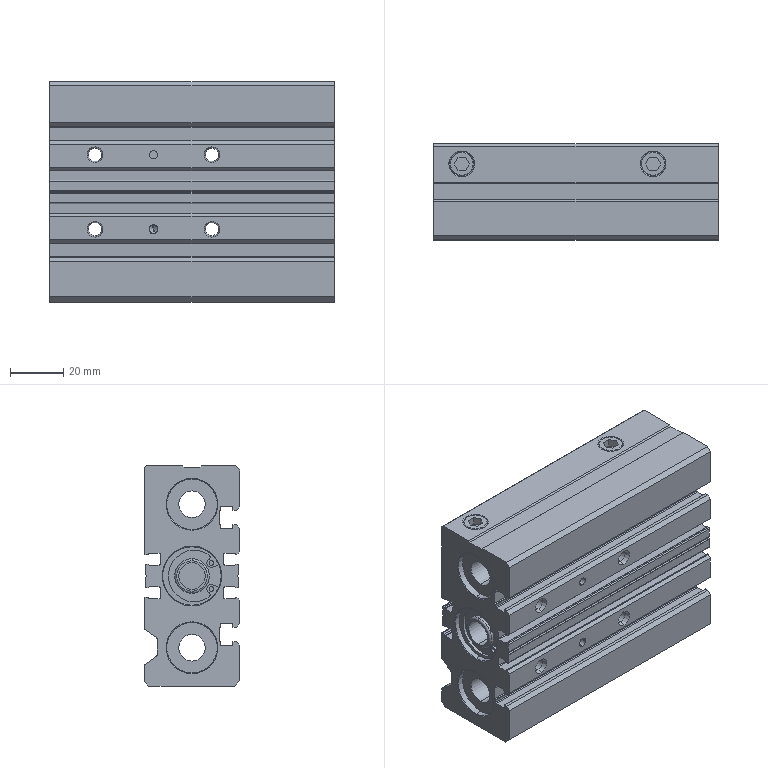Part | STEP file | TC_L_20x7070_b | 1 solid | 377 faces | box 107 x 36 x 83 mm | volume 222327 mm3 | cylinder 170 | plane 135 | cone 70 | torus 2 | commonest cylinder face diameters 0.8 x20 0.4 x18 3 x14 1.8 x12 0.6 x10 1.5 x10